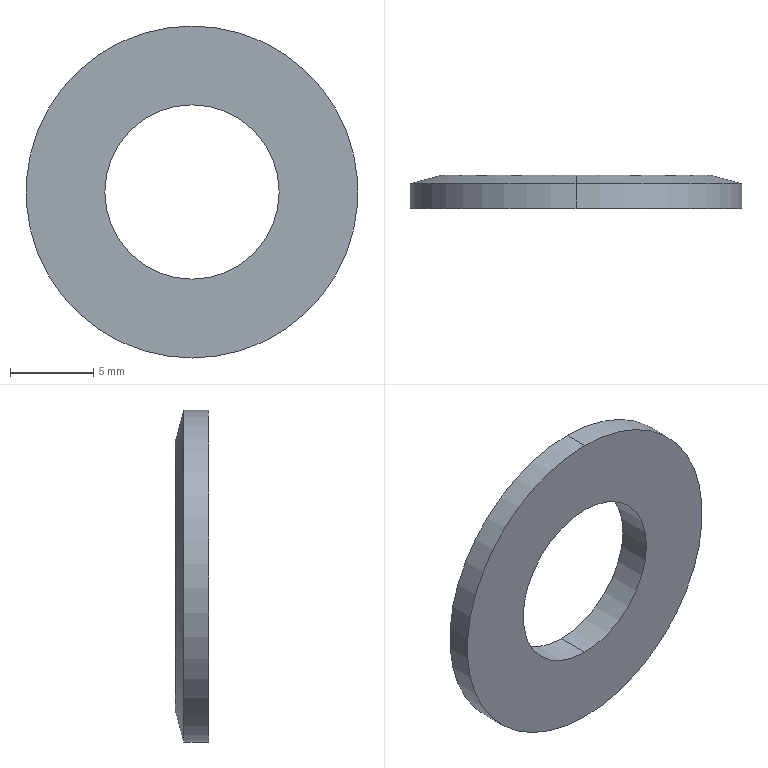Part | SolidWorks | 1 solid | 8 faces | box 20 x 2 x 20 mm | volume 427.568 mm3 | cylinder 4 | cone 2 | plane 2 | commonest cylinder face diameters 10.5 x2 20 x2
STEP:
#1=CARTESIAN_POINT('',(0.,10.145,-10.));
#2=VERTEX_POINT('',#1);
#3=CARTESIAN_POINT('',(0.,10.145,10.));
#4=VERTEX_POINT('',#3);
#5=CARTESIAN_POINT('',(0.,10.145,0.));
#6=DIRECTION('',(0.,-1.,0.));
#7=DIRECTION('',(0.,0.,-1.));
#8=AXIS2_PLACEMENT_3D('',#5,#6,#7);
#9=CIRCLE('',#8,10.);
#10=EDGE_CURVE('',#2,#4,#9,.T.);
#11=ORIENTED_EDGE('',*,*,#10,.T.);
#12=CARTESIAN_POINT('',(0.,8.645,10.));
#13=VERTEX_POINT('',#12);
#14=CARTESIAN_POINT('',(0.,0.,10.));
#15=DIRECTION('',(0.,-1.,0.));
#16=VECTOR('',#15,1000.);
#17=LINE('',#14,#16);
#18=EDGE_CURVE('',#4,#13,#17,.T.);
#19=ORIENTED_EDGE('',*,*,#18,.T.);
#20=CARTESIAN_POINT('',(0.,8.645,-10.));
#21=VERTEX_POINT('',#20);
#22=CARTESIAN_POINT('',(0.,8.645,0.));
#23=DIRECTION('',(0.,-1.,0.));
#24=DIRECTION('',(0.,0.,-1.));
#25=AXIS2_PLACEMENT_3D('',#22,#23,#24);
#26=CIRCLE('',#25,10.);
#27=EDGE_CURVE('',#21,#13,#26,.T.);
#28=ORIENTED_EDGE('',*,*,#27,.F.);
#29=CARTESIAN_POINT('',(0.,0.,-10.));
#30=DIRECTION('',(0.,-1.,0.));
#31=VECTOR('',#30,1000.);
#32=LINE('',#29,#31);
#33=EDGE_CURVE('',#2,#21,#32,.T.);
#34=ORIENTED_EDGE('',*,*,#33,.F.);
#35=EDGE_LOOP('',(#11,#19,#28,#34));
#36=FACE_OUTER_BOUND('',#35,.T.);
#37=CARTESIAN_POINT('',(0.,0.,0.));
#38=DIRECTION('',(0.,-1.,0.));
#39=DIRECTION('',(0.,0.,-1.));
#40=AXIS2_PLACEMENT_3D('',#37,#38,#39);
#41=CYLINDRICAL_SURFACE('',#40,10.);
#42=ADVANCED_FACE('',(#36),#41,.T.);
#43=CARTESIAN_POINT('',(0.,10.645,-8.128));
#44=VERTEX_POINT('',#43);
#45=CARTESIAN_POINT('',(0.,10.645,8.128));
#46=VERTEX_POINT('',#45);
#47=CARTESIAN_POINT('',(0.,10.645,0.));
#48=DIRECTION('',(0.,-1.,0.));
#49=DIRECTION('',(0.,0.,-1.));
#50=AXIS2_PLACEMENT_3D('',#47,#48,#49);
#51=CIRCLE('',#50,8.128);
#52=EDGE_CURVE('',#44,#46,#51,.T.);
#53=ORIENTED_EDGE('',*,*,#52,.T.);
#54=CARTESIAN_POINT('',(0.,10.645,8.128));
#55=DIRECTION('',(0.,-0.258,0.9661));
#56=VECTOR('',#55,1000.);
#57=LINE('',#54,#56);
#58=EDGE_CURVE('',#46,#4,#57,.T.);
#59=ORIENTED_EDGE('',*,*,#58,.T.);
#60=ORIENTED_EDGE('',*,*,#10,.F.);
#61=CARTESIAN_POINT('',(0.,10.645,-8.128));
#62=DIRECTION('',(0.,-0.258,-0.9661));
#63=VECTOR('',#62,1000.);
#64=LINE('',#61,#63);
#65=EDGE_CURVE('',#44,#2,#64,.T.);
#66=ORIENTED_EDGE('',*,*,#65,.F.);
#67=EDGE_LOOP('',(#53,#59,#60,#66));
#68=FACE_OUTER_BOUND('',#67,.T.);
#69=CARTESIAN_POINT('',(0.,10.645,0.));
#70=DIRECTION('',(0.,-1.,0.));
#71=DIRECTION('',(0.,0.,-1.));
#72=AXIS2_PLACEMENT_3D('',#69,#70,#71);
#73=CONICAL_SURFACE('',#72,8.128,1.31);
#74=ADVANCED_FACE('',(#68),#73,.T.);
#75=CARTESIAN_POINT('',(0.,10.645,5.25));
#76=VERTEX_POINT('',#75);
#77=CARTESIAN_POINT('',(0.,10.645,-5.25));
#78=VERTEX_POINT('',#77);
#79=CARTESIAN_POINT('',(0.,10.645,0.));
#80=DIRECTION('',(0.,-1.,0.));
#81=DIRECTION('',(0.,0.,-1.));
#82=AXIS2_PLACEMENT_3D('',#79,#80,#81);
#83=CIRCLE('',#82,5.25);
#84=EDGE_CURVE('',#76,#78,#83,.T.);
#85=ORIENTED_EDGE('',*,*,#84,.F.);
#86=CARTESIAN_POINT('',(0.,8.645,5.25));
#87=VERTEX_POINT('',#86);
#88=CARTESIAN_POINT('',(0.,0.,5.25));
#89=DIRECTION('',(0.,-1.,0.));
#90=VECTOR('',#89,1000.);
#91=LINE('',#88,#90);
#92=EDGE_CURVE('',#76,#87,#91,.T.);
#93=ORIENTED_EDGE('',*,*,#92,.T.);
#94=CARTESIAN_POINT('',(0.,8.645,-5.25));
#95=VERTEX_POINT('',#94);
#96=CARTESIAN_POINT('',(0.,8.645,0.));
#97=DIRECTION('',(0.,-1.,0.));
#98=DIRECTION('',(0.,0.,-1.));
#99=AXIS2_PLACEMENT_3D('',#96,#97,#98);
#100=CIRCLE('',#99,5.25);
#101=EDGE_CURVE('',#87,#95,#100,.T.);
#102=ORIENTED_EDGE('',*,*,#101,.T.);
#103=CARTESIAN_POINT('',(0.,0.,-5.25));
#104=DIRECTION('',(0.,-1.,0.));
#105=VECTOR('',#104,1000.);
#106=LINE('',#103,#105);
#107=EDGE_CURVE('',#78,#95,#106,.T.);
#108=ORIENTED_EDGE('',*,*,#107,.F.);
#109=EDGE_LOOP('',(#85,#93,#102,#108));
#110=FACE_OUTER_BOUND('',#109,.T.);
#111=CARTESIAN_POINT('',(0.,0.,0.));
#112=DIRECTION('',(0.,-1.,0.));
#113=DIRECTION('',(0.,0.,-1.));
#114=AXIS2_PLACEMENT_3D('',#111,#112,#113);
#115=CYLINDRICAL_SURFACE('',#114,5.25);
#116=ADVANCED_FACE('',(#110),#115,.F.);
#117=ORIENTED_EDGE('',*,*,#92,.F.);
#118=CARTESIAN_POINT('',(0.,10.645,0.));
#119=DIRECTION('',(0.,-1.,0.));
#120=DIRECTION('',(0.,0.,-1.));
#121=AXIS2_PLACEMENT_3D('',#118,#119,#120);
#122=CIRCLE('',#121,5.25);
#123=EDGE_CURVE('',#78,#76,#122,.T.);
#124=ORIENTED_EDGE('',*,*,#123,.F.);
#125=ORIENTED_EDGE('',*,*,#107,.T.);
#126=CARTESIAN_POINT('',(0.,8.645,0.));
#127=DIRECTION('',(0.,-1.,0.));
#128=DIRECTION('',(0.,0.,-1.));
#129=AXIS2_PLACEMENT_3D('',#126,#127,#128);
#130=CIRCLE('',#129,5.25);
#131=EDGE_CURVE('',#95,#87,#130,.T.);
#132=ORIENTED_EDGE('',*,*,#131,.T.);
#133=EDGE_LOOP('',(#117,#124,#125,#132));
#134=FACE_OUTER_BOUND('',#133,.T.);
#135=CARTESIAN_POINT('',(0.,0.,0.));
#136=DIRECTION('',(0.,-1.,0.));
#137=DIRECTION('',(0.,0.,-1.));
#138=AXIS2_PLACEMENT_3D('',#135,#136,#137);
#139=CYLINDRICAL_SURFACE('',#138,5.25);
#140=ADVANCED_FACE('',(#134),#139,.F.);
#141=ORIENTED_EDGE('',*,*,#52,.F.);
#142=CARTESIAN_POINT('',(0.,10.645,0.));
#143=DIRECTION('',(0.,-1.,0.));
#144=DIRECTION('',(0.,0.,-1.));
#145=AXIS2_PLACEMENT_3D('',#142,#143,#144);
#146=CIRCLE('',#145,8.128);
#147=EDGE_CURVE('',#46,#44,#146,.T.);
#148=ORIENTED_EDGE('',*,*,#147,.F.);
#149=EDGE_LOOP('',(#141,#148));
#150=FACE_OUTER_BOUND('',#149,.T.);
#151=ORIENTED_EDGE('',*,*,#123,.T.);
#152=ORIENTED_EDGE('',*,*,#84,.T.);
#153=EDGE_LOOP('',(#151,#152));
#154=FACE_BOUND('',#153,.T.);
#155=CARTESIAN_POINT('',(-5.25,10.645,0.));
#156=DIRECTION('',(0.,-1.,0.));
#157=DIRECTION('',(0.,0.,-1.));
#158=AXIS2_PLACEMENT_3D('',#155,#156,#157);
#159=PLANE('',#158);
#160=ADVANCED_FACE('',(#150,#154),#159,.F.);
#161=ORIENTED_EDGE('',*,*,#58,.F.);
#162=ORIENTED_EDGE('',*,*,#147,.T.);
#163=ORIENTED_EDGE('',*,*,#65,.T.);
#164=CARTESIAN_POINT('',(0.,10.145,0.));
#165=DIRECTION('',(0.,-1.,0.));
#166=DIRECTION('',(0.,0.,-1.));
#167=AXIS2_PLACEMENT_3D('',#164,#165,#166);
#168=CIRCLE('',#167,10.);
#169=EDGE_CURVE('',#4,#2,#168,.T.);
#170=ORIENTED_EDGE('',*,*,#169,.F.);
#171=EDGE_LOOP('',(#161,#162,#163,#170));
#172=FACE_OUTER_BOUND('',#171,.T.);
#173=CARTESIAN_POINT('',(0.,10.645,0.));
#174=DIRECTION('',(0.,-1.,0.));
#175=DIRECTION('',(0.,0.,-1.));
#176=AXIS2_PLACEMENT_3D('',#173,#174,#175);
#177=CONICAL_SURFACE('',#176,8.128,1.31);
#178=ADVANCED_FACE('',(#172),#177,.T.);
#179=ORIENTED_EDGE('',*,*,#18,.F.);
#180=ORIENTED_EDGE('',*,*,#169,.T.);
#181=ORIENTED_EDGE('',*,*,#33,.T.);
#182=CARTESIAN_POINT('',(0.,8.645,0.));
#183=DIRECTION('',(0.,-1.,0.));
#184=DIRECTION('',(0.,0.,-1.));
#185=AXIS2_PLACEMENT_3D('',#182,#183,#184);
#186=CIRCLE('',#185,10.);
#187=EDGE_CURVE('',#13,#21,#186,.T.);
#188=ORIENTED_EDGE('',*,*,#187,.F.);
#189=EDGE_LOOP('',(#179,#180,#181,#188));
#190=FACE_OUTER_BOUND('',#189,.T.);
#191=CARTESIAN_POINT('',(0.,0.,0.));
#192=DIRECTION('',(0.,-1.,0.));
#193=DIRECTION('',(0.,0.,-1.));
#194=AXIS2_PLACEMENT_3D('',#191,#192,#193);
#195=CYLINDRICAL_SURFACE('',#194,10.);
#196=ADVANCED_FACE('',(#190),#195,.T.);
#197=ORIENTED_EDGE('',*,*,#131,.F.);
#198=ORIENTED_EDGE('',*,*,#101,.F.);
#199=EDGE_LOOP('',(#197,#198));
#200=FACE_BOUND('',#199,.T.);
#201=ORIENTED_EDGE('',*,*,#27,.T.);
#202=ORIENTED_EDGE('',*,*,#187,.T.);
#203=EDGE_LOOP('',(#201,#202));
#204=FACE_OUTER_BOUND('',#203,.T.);
#205=CARTESIAN_POINT('',(-5.25,8.645,0.));
#206=DIRECTION('',(0.,1.,0.));
#207=DIRECTION('',(0.,0.,1.));
#208=AXIS2_PLACEMENT_3D('',#205,#206,#207);
#209=PLANE('',#208);
#210=ADVANCED_FACE('',(#200,#204),#209,.F.);
#211=CLOSED_SHELL('',(#42,#74,#116,#140,#160,#178,#196,#210));
#212=MANIFOLD_SOLID_BREP('',#211);
#213=CARTESIAN_POINT('',(0.,0.,0.));
#214=DIRECTION('',(0.,0.,1.));
#215=DIRECTION('',(1.,0.,0.));
#216=AXIS2_PLACEMENT_3D('',#213,#214,#215);
#217=(LENGTH_UNIT()NAMED_UNIT(*)SI_UNIT(.MILLI.,.METRE.));
#218=UNCERTAINTY_MEASURE_WITH_UNIT(LENGTH_MEASURE(0.00001),#217,'','');
#219=(NAMED_UNIT(*)PLANE_ANGLE_UNIT()SI_UNIT($,.RADIAN.));
#220=(NAMED_UNIT(*)SI_UNIT($,.STERADIAN.)SOLID_ANGLE_UNIT());
#221=(GEOMETRIC_REPRESENTATION_CONTEXT(3)GLOBAL_UNCERTAINTY_ASSIGNED_CONTEXT((#218))GLOBAL_UNIT_ASSIGNED_CONTEXT((#217,#219,#220))REPRESENTATION_CONTEXT('',''));
#222=ADVANCED_BREP_SHAPE_REPRESENTATION('',(#212,#216),#221);